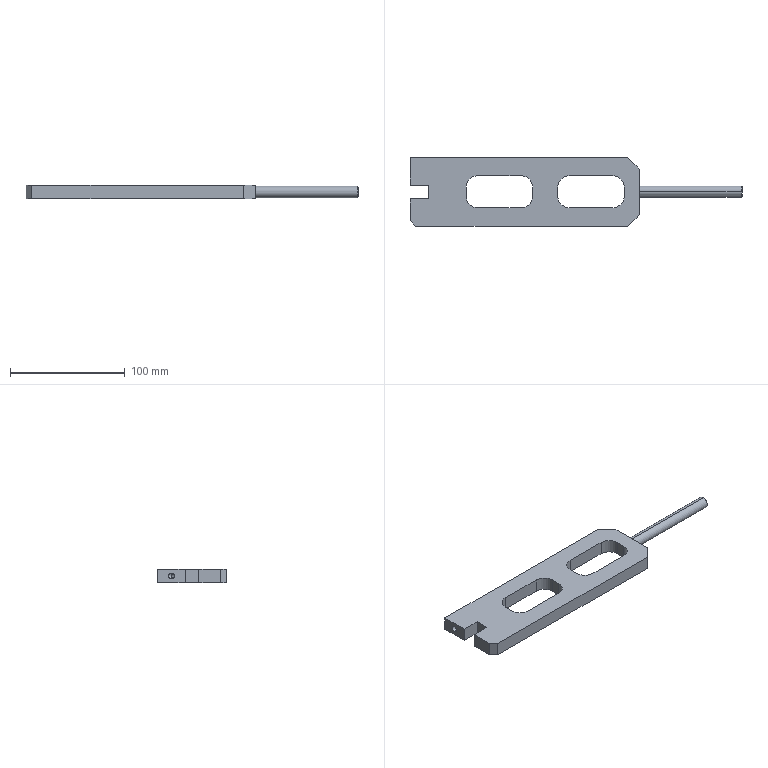Part | SolidWorks | features Chamfer 3, ICE 3, HoleWzd 2, Extrusion 1, Fillet 1, Revolution 1 | 1 solid | 41 faces | box 289.75 x 60 x 12 mm | volume 104525 mm3 | plane 21 | cylinder 14 | cone 6 | commonest cylinder face diameters 20 x8 5 x2 8.5 x2 10 x2
STEP:
#1=CARTESIAN_POINT('',(90.5,0.2,4.25));
#2=VERTEX_POINT('',#1);
#3=CARTESIAN_POINT('',(90.5,0.2,-4.25));
#4=VERTEX_POINT('',#3);
#5=CARTESIAN_POINT('',(90.5,0.2,0.));
#6=DIRECTION('',(1.,0.,0.));
#7=DIRECTION('',(0.,0.,-1.));
#8=AXIS2_PLACEMENT_3D('',#5,#6,#7);
#9=CIRCLE('',#8,4.25);
#10=EDGE_CURVE('',#2,#4,#9,.T.);
#11=ORIENTED_EDGE('',*,*,#10,.F.);
#12=CARTESIAN_POINT('',(189.75,0.2,4.25));
#13=VERTEX_POINT('',#12);
#14=CARTESIAN_POINT('',(190.,0.2,4.25));
#15=DIRECTION('',(1.,0.,0.));
#16=VECTOR('',#15,1000.);
#17=LINE('',#14,#16);
#18=EDGE_CURVE('',#2,#13,#17,.T.);
#19=ORIENTED_EDGE('',*,*,#18,.T.);
#20=CARTESIAN_POINT('',(189.75,0.2,-4.25));
#21=VERTEX_POINT('',#20);
#22=CARTESIAN_POINT('',(189.75,0.2,0.));
#23=DIRECTION('',(1.,0.,0.));
#24=DIRECTION('',(0.,0.,1.));
#25=AXIS2_PLACEMENT_3D('',#22,#23,#24);
#26=CIRCLE('',#25,4.25);
#27=EDGE_CURVE('',#13,#21,#26,.T.);
#28=ORIENTED_EDGE('',*,*,#27,.T.);
#29=CARTESIAN_POINT('',(190.,0.2,-4.25));
#30=DIRECTION('',(1.,0.,0.));
#31=VECTOR('',#30,1000.);
#32=LINE('',#29,#31);
#33=EDGE_CURVE('',#4,#21,#32,.T.);
#34=ORIENTED_EDGE('',*,*,#33,.F.);
#35=EDGE_LOOP('',(#11,#19,#28,#34));
#36=FACE_OUTER_BOUND('',#35,.T.);
#37=CARTESIAN_POINT('',(190.,0.2,0.));
#38=DIRECTION('',(1.,0.,0.));
#39=DIRECTION('',(0.,0.,-1.));
#40=AXIS2_PLACEMENT_3D('',#37,#38,#39);
#41=CYLINDRICAL_SURFACE('',#40,4.25);
#42=ADVANCED_FACE('',(#36),#41,.F.);
#43=CARTESIAN_POINT('',(87.946,0.2,0.));
#44=VERTEX_POINT('',#43);
#45=CARTESIAN_POINT('',(90.5,0.2,-4.25));
#46=DIRECTION('',(0.515,0.,-0.8572));
#47=VECTOR('',#46,1000.);
#48=LINE('',#45,#47);
#49=EDGE_CURVE('',#44,#4,#48,.T.);
#50=ORIENTED_EDGE('',*,*,#49,.F.);
#51=CARTESIAN_POINT('',(90.5,0.2,4.25));
#52=DIRECTION('',(0.515,0.,0.8572));
#53=VECTOR('',#52,1000.);
#54=LINE('',#51,#53);
#55=EDGE_CURVE('',#44,#2,#54,.T.);
#56=ORIENTED_EDGE('',*,*,#55,.T.);
#57=ORIENTED_EDGE('',*,*,#10,.T.);
#58=EDGE_LOOP('',(#50,#56,#57));
#59=FACE_OUTER_BOUND('',#58,.T.);
#60=CARTESIAN_POINT('',(90.5,0.2,0.));
#61=DIRECTION('',(1.,0.,0.));
#62=DIRECTION('',(0.,0.,-1.));
#63=AXIS2_PLACEMENT_3D('',#60,#61,#62);
#64=CONICAL_SURFACE('',#63,4.25,1.03);
#65=ADVANCED_FACE('',(#59),#64,.F.);
#66=CARTESIAN_POINT('',(189.75,0.2,0.));
#67=DIRECTION('',(1.,0.,0.));
#68=DIRECTION('',(0.,0.,1.));
#69=AXIS2_PLACEMENT_3D('',#66,#67,#68);
#70=CIRCLE('',#69,4.25);
#71=EDGE_CURVE('',#21,#13,#70,.T.);
#72=ORIENTED_EDGE('',*,*,#71,.F.);
#73=CARTESIAN_POINT('',(189.,0.2,-5.));
#74=VERTEX_POINT('',#73);
#75=CARTESIAN_POINT('',(189.,0.2,-5.));
#76=DIRECTION('',(-0.7071,0.,-0.7071));
#77=VECTOR('',#76,1000.);
#78=LINE('',#75,#77);
#79=EDGE_CURVE('',#21,#74,#78,.T.);
#80=ORIENTED_EDGE('',*,*,#79,.T.);
#81=CARTESIAN_POINT('',(189.,0.2,5.));
#82=VERTEX_POINT('',#81);
#83=CARTESIAN_POINT('',(189.,0.2,0.));
#84=DIRECTION('',(-1.,0.,0.));
#85=DIRECTION('',(0.,0.,-1.));
#86=AXIS2_PLACEMENT_3D('',#83,#84,#85);
#87=CIRCLE('',#86,5.);
#88=EDGE_CURVE('',#82,#74,#87,.T.);
#89=ORIENTED_EDGE('',*,*,#88,.F.);
#90=CARTESIAN_POINT('',(189.,0.2,5.));
#91=DIRECTION('',(-0.7071,0.,0.7071));
#92=VECTOR('',#91,1000.);
#93=LINE('',#90,#92);
#94=EDGE_CURVE('',#13,#82,#93,.T.);
#95=ORIENTED_EDGE('',*,*,#94,.F.);
#96=EDGE_LOOP('',(#72,#80,#89,#95));
#97=FACE_OUTER_BOUND('',#96,.T.);
#98=CARTESIAN_POINT('',(189.,0.2,0.));
#99=DIRECTION('',(-1.,0.,0.));
#100=DIRECTION('',(0.,0.,1.));
#101=AXIS2_PLACEMENT_3D('',#98,#99,#100);
#102=CONICAL_SURFACE('',#101,5.,0.7854);
#103=ADVANCED_FACE('',(#97),#102,.T.);
#104=CARTESIAN_POINT('',(-87.,18.,-2.5));
#105=VERTEX_POINT('',#104);
#106=CARTESIAN_POINT('',(-87.,18.,2.5));
#107=VERTEX_POINT('',#106);
#108=CARTESIAN_POINT('',(-87.,18.,0.));
#109=DIRECTION('',(-1.,0.,0.));
#110=DIRECTION('',(0.,0.,1.));
#111=AXIS2_PLACEMENT_3D('',#108,#109,#110);
#112=CIRCLE('',#111,2.5);
#113=EDGE_CURVE('',#105,#107,#112,.T.);
#114=ORIENTED_EDGE('',*,*,#113,.F.);
#115=CARTESIAN_POINT('',(-100.,18.,-2.5));
#116=VERTEX_POINT('',#115);
#117=CARTESIAN_POINT('',(-100.,18.,-2.5));
#118=DIRECTION('',(-1.,0.,0.));
#119=VECTOR('',#118,1000.);
#120=LINE('',#117,#119);
#121=EDGE_CURVE('',#105,#116,#120,.T.);
#122=ORIENTED_EDGE('',*,*,#121,.T.);
#123=CARTESIAN_POINT('',(-100.,18.,2.5));
#124=VERTEX_POINT('',#123);
#125=CARTESIAN_POINT('',(-100.,18.,0.));
#126=DIRECTION('',(-1.,0.,0.));
#127=DIRECTION('',(0.,0.,1.));
#128=AXIS2_PLACEMENT_3D('',#125,#126,#127);
#129=CIRCLE('',#128,2.5);
#130=EDGE_CURVE('',#116,#124,#129,.T.);
#131=ORIENTED_EDGE('',*,*,#130,.T.);
#132=CARTESIAN_POINT('',(-100.,18.,2.5));
#133=DIRECTION('',(-1.,0.,0.));
#134=VECTOR('',#133,1000.);
#135=LINE('',#132,#134);
#136=EDGE_CURVE('',#107,#124,#135,.T.);
#137=ORIENTED_EDGE('',*,*,#136,.F.);
#138=EDGE_LOOP('',(#114,#122,#131,#137));
#139=FACE_OUTER_BOUND('',#138,.T.);
#140=CARTESIAN_POINT('',(-100.,18.,0.));
#141=DIRECTION('',(-1.,0.,0.));
#142=DIRECTION('',(0.,0.,1.));
#143=AXIS2_PLACEMENT_3D('',#140,#141,#142);
#144=CYLINDRICAL_SURFACE('',#143,2.5);
#145=ADVANCED_FACE('',(#139),#144,.F.);
#146=CARTESIAN_POINT('',(-85.498,18.,0.));
#147=VERTEX_POINT('',#146);
#148=CARTESIAN_POINT('',(-87.,18.,2.5));
#149=DIRECTION('',(-0.515,0.,0.8572));
#150=VECTOR('',#149,1000.);
#151=LINE('',#148,#150);
#152=EDGE_CURVE('',#147,#107,#151,.T.);
#153=ORIENTED_EDGE('',*,*,#152,.F.);
#154=CARTESIAN_POINT('',(-87.,18.,-2.5));
#155=DIRECTION('',(-0.515,0.,-0.8572));
#156=VECTOR('',#155,1000.);
#157=LINE('',#154,#156);
#158=EDGE_CURVE('',#147,#105,#157,.T.);
#159=ORIENTED_EDGE('',*,*,#158,.T.);
#160=ORIENTED_EDGE('',*,*,#113,.T.);
#161=EDGE_LOOP('',(#153,#159,#160));
#162=FACE_OUTER_BOUND('',#161,.T.);
#163=CARTESIAN_POINT('',(-87.,18.,0.));
#164=DIRECTION('',(-1.,0.,0.));
#165=DIRECTION('',(0.,0.,1.));
#166=AXIS2_PLACEMENT_3D('',#163,#164,#165);
#167=CONICAL_SURFACE('',#166,2.5,1.03);
#168=ADVANCED_FACE('',(#162),#167,.F.);
#169=ORIENTED_EDGE('',*,*,#88,.T.);
#170=CARTESIAN_POINT('',(100.,0.2,-5.));
#171=VERTEX_POINT('',#170);
#172=CARTESIAN_POINT('',(190.,0.2,-5.));
#173=DIRECTION('',(-1.,0.,0.));
#174=VECTOR('',#173,1000.);
#175=LINE('',#172,#174);
#176=EDGE_CURVE('',#74,#171,#175,.T.);
#177=ORIENTED_EDGE('',*,*,#176,.T.);
#178=CARTESIAN_POINT('',(100.,0.2,5.));
#179=VERTEX_POINT('',#178);
#180=CARTESIAN_POINT('',(100.,0.2,0.));
#181=DIRECTION('',(-1.,0.,0.));
#182=DIRECTION('',(0.,0.,1.));
#183=AXIS2_PLACEMENT_3D('',#180,#181,#182);
#184=CIRCLE('',#183,5.);
#185=EDGE_CURVE('',#179,#171,#184,.T.);
#186=ORIENTED_EDGE('',*,*,#185,.F.);
#187=CARTESIAN_POINT('',(190.,0.2,5.));
#188=DIRECTION('',(-1.,0.,0.));
#189=VECTOR('',#188,1000.);
#190=LINE('',#187,#189);
#191=EDGE_CURVE('',#82,#179,#190,.T.);
#192=ORIENTED_EDGE('',*,*,#191,.F.);
#193=EDGE_LOOP('',(#169,#177,#186,#192));
#194=FACE_OUTER_BOUND('',#193,.T.);
#195=CARTESIAN_POINT('',(190.,0.2,0.));
#196=DIRECTION('',(-1.,0.,0.));
#197=DIRECTION('',(0.,0.,1.));
#198=AXIS2_PLACEMENT_3D('',#195,#196,#197);
#199=CYLINDRICAL_SURFACE('',#198,5.);
#200=ADVANCED_FACE('',(#194),#199,.T.);
#201=CARTESIAN_POINT('',(-100.,-6.,-6.));
#202=VERTEX_POINT('',#201);
#203=CARTESIAN_POINT('',(-100.,-25.,-6.));
#204=VERTEX_POINT('',#203);
#205=CARTESIAN_POINT('',(-100.,30.,-6.));
#206=DIRECTION('',(0.,-1.,0.));
#207=VECTOR('',#206,1000.);
#208=LINE('',#205,#207);
#209=EDGE_CURVE('',#202,#204,#208,.T.);
#210=ORIENTED_EDGE('',*,*,#209,.T.);
#211=CARTESIAN_POINT('',(-100.,-25.,6.));
#212=VERTEX_POINT('',#211);
#213=CARTESIAN_POINT('',(-100.,-25.,-6.));
#214=DIRECTION('',(0.,0.,1.));
#215=VECTOR('',#214,1000.);
#216=LINE('',#213,#215);
#217=EDGE_CURVE('',#204,#212,#216,.T.);
#218=ORIENTED_EDGE('',*,*,#217,.T.);
#219=CARTESIAN_POINT('',(-100.,-6.,6.));
#220=VERTEX_POINT('',#219);
#221=CARTESIAN_POINT('',(-100.,30.,6.));
#222=DIRECTION('',(0.,-1.,0.));
#223=VECTOR('',#222,1000.);
#224=LINE('',#221,#223);
#225=EDGE_CURVE('',#220,#212,#224,.T.);
#226=ORIENTED_EDGE('',*,*,#225,.F.);
#227=CARTESIAN_POINT('',(-100.,-6.,6.));
#228=DIRECTION('',(0.,0.,-1.));
#229=VECTOR('',#228,1000.);
#230=LINE('',#227,#229);
#231=EDGE_CURVE('',#220,#202,#230,.T.);
#232=ORIENTED_EDGE('',*,*,#231,.T.);
#233=EDGE_LOOP('',(#210,#218,#226,#232));
#234=FACE_OUTER_BOUND('',#233,.T.);
#235=CARTESIAN_POINT('',(-100.,30.,-6.));
#236=DIRECTION('',(-1.,0.,0.));
#237=DIRECTION('',(0.,0.,1.));
#238=AXIS2_PLACEMENT_3D('',#235,#236,#237);
#239=PLANE('',#238);
#240=ADVANCED_FACE('',(#234),#239,.T.);
#241=CARTESIAN_POINT('',(90.,30.,6.));
#242=VERTEX_POINT('',#241);
#243=CARTESIAN_POINT('',(-100.,30.,6.));
#244=VERTEX_POINT('',#243);
#245=CARTESIAN_POINT('',(100.,30.,6.));
#246=DIRECTION('',(-1.,0.,0.));
#247=VECTOR('',#246,1000.);
#248=LINE('',#245,#247);
#249=EDGE_CURVE('',#242,#244,#248,.T.);
#250=ORIENTED_EDGE('',*,*,#249,.F.);
#251=CARTESIAN_POINT('',(90.,30.,-6.));
#252=VERTEX_POINT('',#251);
#253=CARTESIAN_POINT('',(90.,30.,-6.));
#254=DIRECTION('',(0.,0.,-1.));
#255=VECTOR('',#254,1000.);
#256=LINE('',#253,#255);
#257=EDGE_CURVE('',#242,#252,#256,.T.);
#258=ORIENTED_EDGE('',*,*,#257,.T.);
#259=CARTESIAN_POINT('',(-100.,30.,-6.));
#260=VERTEX_POINT('',#259);
#261=CARTESIAN_POINT('',(100.,30.,-6.));
#262=DIRECTION('',(-1.,0.,0.));
#263=VECTOR('',#262,1000.);
#264=LINE('',#261,#263);
#265=EDGE_CURVE('',#252,#260,#264,.T.);
#266=ORIENTED_EDGE('',*,*,#265,.T.);
#267=CARTESIAN_POINT('',(-100.,30.,-6.));
#268=DIRECTION('',(0.,0.,1.));
#269=VECTOR('',#268,1000.);
#270=LINE('',#267,#269);
#271=EDGE_CURVE('',#260,#244,#270,.T.);
#272=ORIENTED_EDGE('',*,*,#271,.T.);
#273=EDGE_LOOP('',(#250,#258,#266,#272));
#274=FACE_OUTER_BOUND('',#273,.T.);
#275=CARTESIAN_POINT('',(100.,30.,-6.));
#276=DIRECTION('',(0.,1.,0.));
#277=DIRECTION('',(0.,0.,1.));
#278=AXIS2_PLACEMENT_3D('',#275,#276,#277);
#279=PLANE('',#278);
#280=ADVANCED_FACE('',(#274),#279,.T.);
#281=ORIENTED_EDGE('',*,*,#185,.T.);
#282=CARTESIAN_POINT('',(100.,0.2,0.));
#283=DIRECTION('',(-1.,0.,0.));
#284=DIRECTION('',(0.,0.,1.));
#285=AXIS2_PLACEMENT_3D('',#282,#283,#284);
#286=CIRCLE('',#285,5.);
#287=EDGE_CURVE('',#171,#179,#286,.T.);
#288=ORIENTED_EDGE('',*,*,#287,.T.);
#289=EDGE_LOOP('',(#281,#288));
#290=FACE_BOUND('',#289,.T.);
#291=CARTESIAN_POINT('',(100.,-20.,-6.));
#292=VERTEX_POINT('',#291);
#293=CARTESIAN_POINT('',(100.,20.,-6.));
#294=VERTEX_POINT('',#293);
#295=CARTESIAN_POINT('',(100.,-30.,-6.));
#296=DIRECTION('',(0.,1.,0.));
#297=VECTOR('',#296,1000.);
#298=LINE('',#295,#297);
#299=EDGE_CURVE('',#292,#294,#298,.T.);
#300=ORIENTED_EDGE('',*,*,#299,.T.);
#301=CARTESIAN_POINT('',(100.,20.,6.));
#302=VERTEX_POINT('',#301);
#303=CARTESIAN_POINT('',(100.,20.,-6.));
#304=DIRECTION('',(0.,0.,1.));
#305=VECTOR('',#304,1000.);
#306=LINE('',#303,#305);
#307=EDGE_CURVE('',#294,#302,#306,.T.);
#308=ORIENTED_EDGE('',*,*,#307,.T.);
#309=CARTESIAN_POINT('',(100.,-20.,6.));
#310=VERTEX_POINT('',#309);
#311=CARTESIAN_POINT('',(100.,-30.,6.));
#312=DIRECTION('',(0.,1.,0.));
#313=VECTOR('',#312,1000.);
#314=LINE('',#311,#313);
#315=EDGE_CURVE('',#310,#302,#314,.T.);
#316=ORIENTED_EDGE('',*,*,#315,.F.);
#317=CARTESIAN_POINT('',(100.,-20.,-6.));
#318=DIRECTION('',(0.,0.,-1.));
#319=VECTOR('',#318,1000.);
#320=LINE('',#317,#319);
#321=EDGE_CURVE('',#310,#292,#320,.T.);
#322=ORIENTED_EDGE('',*,*,#321,.T.);
#323=EDGE_LOOP('',(#300,#308,#316,#322));
#324=FACE_OUTER_BOUND('',#323,.T.);
#325=CARTESIAN_POINT('',(100.,-30.,-6.));
#326=DIRECTION('',(1.,0.,0.));
#327=DIRECTION('',(0.,0.,-1.));
#328=AXIS2_PLACEMENT_3D('',#325,#326,#327);
#329=PLANE('',#328);
#330=ADVANCED_FACE('',(#290,#324),#329,.T.);
#331=CARTESIAN_POINT('',(-95.,-30.,6.));
#332=VERTEX_POINT('',#331);
#333=CARTESIAN_POINT('',(90.,-30.,6.));
#334=VERTEX_POINT('',#333);
#335=CARTESIAN_POINT('',(-100.,-30.,6.));
#336=DIRECTION('',(1.,0.,0.));
#337=VECTOR('',#336,1000.);
#338=LINE('',#335,#337);
#339=EDGE_CURVE('',#332,#334,#338,.T.);
#340=ORIENTED_EDGE('',*,*,#339,.F.);
#341=CARTESIAN_POINT('',(-95.,-30.,-6.));
#342=VERTEX_POINT('',#341);
#343=CARTESIAN_POINT('',(-95.,-30.,-6.));
#344=DIRECTION('',(0.,0.,-1.));
#345=VECTOR('',#344,1000.);
#346=LINE('',#343,#345);
#347=EDGE_CURVE('',#332,#342,#346,.T.);
#348=ORIENTED_EDGE('',*,*,#347,.T.);
#349=CARTESIAN_POINT('',(90.,-30.,-6.));
#350=VERTEX_POINT('',#349);
#351=CARTESIAN_POINT('',(-100.,-30.,-6.));
#352=DIRECTION('',(1.,0.,0.));
#353=VECTOR('',#352,1000.);
#354=LINE('',#351,#353);
#355=EDGE_CURVE('',#342,#350,#354,.T.);
#356=ORIENTED_EDGE('',*,*,#355,.T.);
#357=CARTESIAN_POINT('',(90.,-30.,-6.));
#358=DIRECTION('',(0.,0.,1.));
#359=VECTOR('',#358,1000.);
#360=LINE('',#357,#359);
#361=EDGE_CURVE('',#350,#334,#360,.T.);
#362=ORIENTED_EDGE('',*,*,#361,.T.);
#363=EDGE_LOOP('',(#340,#348,#356,#362));
#364=FACE_OUTER_BOUND('',#363,.T.);
#365=CARTESIAN_POINT('',(-100.,-30.,-6.));
#366=DIRECTION('',(0.,-1.,0.));
#367=DIRECTION('',(0.,0.,-1.));
#368=AXIS2_PLACEMENT_3D('',#365,#366,#367);
#369=PLANE('',#368);
#370=ADVANCED_FACE('',(#364),#369,.T.);
#371=CARTESIAN_POINT('',(-100.,18.,0.));
#372=DIRECTION('',(-1.,0.,0.));
#373=DIRECTION('',(0.,0.,1.));
#374=AXIS2_PLACEMENT_3D('',#371,#372,#373);
#375=CIRCLE('',#374,2.5);
#376=EDGE_CURVE('',#124,#116,#375,.T.);
#377=ORIENTED_EDGE('',*,*,#376,.F.);
#378=ORIENTED_EDGE('',*,*,#130,.F.);
#379=EDGE_LOOP('',(#377,#378));
#380=FACE_BOUND('',#379,.T.);
#381=CARTESIAN_POINT('',(-100.,6.,6.));
#382=VERTEX_POINT('',#381);
#383=CARTESIAN_POINT('',(-100.,6.,-6.));
#384=VERTEX_POINT('',#383);
#385=CARTESIAN_POINT('',(-100.,6.,6.));
#386=DIRECTION('',(0.,0.,-1.));
#387=VECTOR('',#386,1000.);
#388=LINE('',#385,#387);
#389=EDGE_CURVE('',#382,#384,#388,.T.);
#390=ORIENTED_EDGE('',*,*,#389,.F.);
#391=CARTESIAN_POINT('',(-100.,30.,6.));
#392=DIRECTION('',(0.,-1.,0.));
#393=VECTOR('',#392,1000.);
#394=LINE('',#391,#393);
#395=EDGE_CURVE('',#244,#382,#394,.T.);
#396=ORIENTED_EDGE('',*,*,#395,.F.);
#397=ORIENTED_EDGE('',*,*,#271,.F.);
#398=CARTESIAN_POINT('',(-100.,30.,-6.));
#399=DIRECTION('',(0.,-1.,0.));
#400=VECTOR('',#399,1000.);
#401=LINE('',#398,#400);
#402=EDGE_CURVE('',#260,#384,#401,.T.);
#403=ORIENTED_EDGE('',*,*,#402,.T.);
#404=EDGE_LOOP('',(#390,#396,#397,#403));
#405=FACE_OUTER_BOUND('',#404,.T.);
#406=CARTESIAN_POINT('',(-100.,30.,-6.));
#407=DIRECTION('',(-1.,0.,0.));
#408=DIRECTION('',(0.,0.,1.));
#409=AXIS2_PLACEMENT_3D('',#406,#407,#408);
#410=PLANE('',#409);
#411=ADVANCED_FACE('',(#380,#405),#410,.T.);
#412=CARTESIAN_POINT('',(39.,14.2,-6.));
#413=VERTEX_POINT('',#412);
#414=CARTESIAN_POINT('',(77.,14.2,-6.));
#415=VERTEX_POINT('',#414);
#416=CARTESIAN_POINT('',(29.,14.2,-6.));
#417=DIRECTION('',(1.,0.,0.));
#418=VECTOR('',#417,1000.);
#419=LINE('',#416,#418);
#420=EDGE_CURVE('',#413,#415,#419,.T.);
#421=ORIENTED_EDGE('',*,*,#420,.F.);
#422=CARTESIAN_POINT('',(29.,4.2,-6.));
#423=VERTEX_POINT('',#422);
#424=CARTESIAN_POINT('',(39.,4.2,-6.));
#425=DIRECTION('',(0.,0.,1.));
#426=DIRECTION('',(1.,0.,0.));
#427=AXIS2_PLACEMENT_3D('',#424,#425,#426);
#428=CIRCLE('',#427,10.);
#429=EDGE_CURVE('',#413,#423,#428,.T.);
#430=ORIENTED_EDGE('',*,*,#429,.T.);
#431=CARTESIAN_POINT('',(29.,-3.8,-6.));
#432=VERTEX_POINT('',#431);
#433=CARTESIAN_POINT('',(29.,-13.8,-6.));
#434=DIRECTION('',(0.,1.,0.));
#435=VECTOR('',#434,1000.);
#436=LINE('',#433,#435);
#437=EDGE_CURVE('',#432,#423,#436,.T.);
#438=ORIENTED_EDGE('',*,*,#437,.F.);
#439=CARTESIAN_POINT('',(39.,-13.8,-6.));
#440=VERTEX_POINT('',#439);
#441=CARTESIAN_POINT('',(39.,-3.8,-6.));
#442=DIRECTION('',(0.,0.,1.));
#443=DIRECTION('',(1.,0.,0.));
#444=AXIS2_PLACEMENT_3D('',#441,#442,#443);
#445=CIRCLE('',#444,10.);
#446=EDGE_CURVE('',#432,#440,#445,.T.);
#447=ORIENTED_EDGE('',*,*,#446,.T.);
#448=CARTESIAN_POINT('',(77.,-13.8,-6.));
#449=VERTEX_POINT('',#448);
#450=CARTESIAN_POINT('',(87.,-13.8,-6.));
#451=DIRECTION('',(-1.,0.,0.));
#452=VECTOR('',#451,1000.);
#453=LINE('',#450,#452);
#454=EDGE_CURVE('',#449,#440,#453,.T.);
#455=ORIENTED_EDGE('',*,*,#454,.F.);
#456=CARTESIAN_POINT('',(87.,-3.8,-6.));
#457=VERTEX_POINT('',#456);
#458=CARTESIAN_POINT('',(77.,-3.8,-6.));
#459=DIRECTION('',(0.,0.,1.));
#460=DIRECTION('',(1.,0.,0.));
#461=AXIS2_PLACEMENT_3D('',#458,#459,#460);
#462=CIRCLE('',#461,10.);
#463=EDGE_CURVE('',#449,#457,#462,.T.);
#464=ORIENTED_EDGE('',*,*,#463,.T.);
#465=CARTESIAN_POINT('',(87.,4.2,-6.));
#466=VERTEX_POINT('',#465);
#467=CARTESIAN_POINT('',(87.,14.2,-6.));
#468=DIRECTION('',(0.,-1.,0.));
#469=VECTOR('',#468,1000.);
#470=LINE('',#467,#469);
#471=EDGE_CURVE('',#466,#457,#470,.T.);
#472=ORIENTED_EDGE('',*,*,#471,.F.);
#473=CARTESIAN_POINT('',(77.,4.2,-6.));
#474=DIRECTION('',(0.,0.,1.));
#475=DIRECTION('',(1.,0.,0.));
#476=AXIS2_PLACEMENT_3D('',#473,#474,#475);
#477=CIRCLE('',#476,10.);
#478=EDGE_CURVE('',#466,#415,#477,.T.);
#479=ORIENTED_EDGE('',*,*,#478,.T.);
#480=EDGE_LOOP('',(#421,#430,#438,#447,#455,#464,#472,#479));
#481=FACE_BOUND('',#480,.T.);
#482=CARTESIAN_POINT('',(7.,-3.8,-6.));
#483=VERTEX_POINT('',#482);
#484=CARTESIAN_POINT('',(7.,4.2,-6.));
#485=VERTEX_POINT('',#484);
#486=CARTESIAN_POINT('',(7.,-13.8,-6.));
#487=DIRECTION('',(0.,1.,0.));
#488=VECTOR('',#487,1000.);
#489=LINE('',#486,#488);
#490=EDGE_CURVE('',#483,#485,#489,.T.);
#491=ORIENTED_EDGE('',*,*,#490,.T.);
#492=CARTESIAN_POINT('',(-3.,14.2,-6.));
#493=VERTEX_POINT('',#492);
#494=CARTESIAN_POINT('',(-3.,4.2,-6.));
#495=DIRECTION('',(0.,0.,1.));
#496=DIRECTION('',(1.,0.,0.));
#497=AXIS2_PLACEMENT_3D('',#494,#495,#496);
#498=CIRCLE('',#497,10.);
#499=EDGE_CURVE('',#485,#493,#498,.T.);
#500=ORIENTED_EDGE('',*,*,#499,.T.);
#501=CARTESIAN_POINT('',(-41.,14.2,-6.));
#502=VERTEX_POINT('',#501);
#503=CARTESIAN_POINT('',(7.,14.2,-6.));
#504=DIRECTION('',(-1.,0.,0.));
#505=VECTOR('',#504,1000.);
#506=LINE('',#503,#505);
#507=EDGE_CURVE('',#493,#502,#506,.T.);
#508=ORIENTED_EDGE('',*,*,#507,.T.);
#509=CARTESIAN_POINT('',(-51.,4.2,-6.));
#510=VERTEX_POINT('',#509);
#511=CARTESIAN_POINT('',(-41.,4.2,-6.));
#512=DIRECTION('',(0.,0.,1.));
#513=DIRECTION('',(1.,0.,0.));
#514=AXIS2_PLACEMENT_3D('',#511,#512,#513);
#515=CIRCLE('',#514,10.);
#516=EDGE_CURVE('',#502,#510,#515,.T.);
#517=ORIENTED_EDGE('',*,*,#516,.T.);
#518=CARTESIAN_POINT('',(-51.,-3.8,-6.));
#519=VERTEX_POINT('',#518);
#520=CARTESIAN_POINT('',(-51.,14.2,-6.));
#521=DIRECTION('',(0.,-1.,0.));
#522=VECTOR('',#521,1000.);
#523=LINE('',#520,#522);
#524=EDGE_CURVE('',#510,#519,#523,.T.);
#525=ORIENTED_EDGE('',*,*,#524,.T.);
#526=CARTESIAN_POINT('',(-41.,-13.8,-6.));
#527=VERTEX_POINT('',#526);
#528=CARTESIAN_POINT('',(-41.,-3.8,-6.));
#529=DIRECTION('',(0.,0.,1.));
#530=DIRECTION('',(1.,0.,0.));
#531=AXIS2_PLACEMENT_3D('',#528,#529,#530);
#532=CIRCLE('',#531,10.);
#533=EDGE_CURVE('',#519,#527,#532,.T.);
#534=ORIENTED_EDGE('',*,*,#533,.T.);
#535=CARTESIAN_POINT('',(-3.,-13.8,-6.));
#536=VERTEX_POINT('',#535);
#537=CARTESIAN_POINT('',(-51.,-13.8,-6.));
#538=DIRECTION('',(1.,0.,0.));
#539=VECTOR('',#538,1000.);
#540=LINE('',#537,#539);
#541=EDGE_CURVE('',#527,#536,#540,.T.);
#542=ORIENTED_EDGE('',*,*,#541,.T.);
#543=CARTESIAN_POINT('',(-3.,-3.8,-6.));
#544=DIRECTION('',(0.,0.,1.));
#545=DIRECTION('',(1.,0.,0.));
#546=AXIS2_PLACEMENT_3D('',#543,#544,#545);
#547=CIRCLE('',#546,10.);
#548=EDGE_CURVE('',#536,#483,#547,.T.);
#549=ORIENTED_EDGE('',*,*,#548,.T.);
#550=EDGE_LOOP('',(#491,#500,#508,#517,#525,#534,#542,#549));
#551=FACE_BOUND('',#550,.T.);
#552=ORIENTED_EDGE('',*,*,#355,.F.);
#553=CARTESIAN_POINT('',(-100.,-25.,-6.));
#554=DIRECTION('',(-0.7071,0.7071,0.));
#555=VECTOR('',#554,1000.);
#556=LINE('',#553,#555);
#557=EDGE_CURVE('',#342,#204,#556,.T.);
#558=ORIENTED_EDGE('',*,*,#557,.T.);
#559=ORIENTED_EDGE('',*,*,#209,.F.);
#560=CARTESIAN_POINT('',(-84.,-6.,-6.));
#561=VERTEX_POINT('',#560);
#562=CARTESIAN_POINT('',(-84.,-6.,-6.));
#563=DIRECTION('',(-1.,0.,0.));
#564=VECTOR('',#563,1000.);
#565=LINE('',#562,#564);
#566=EDGE_CURVE('',#561,#202,#565,.T.);
#567=ORIENTED_EDGE('',*,*,#566,.F.);
#568=CARTESIAN_POINT('',(-84.,6.,-6.));
#569=VERTEX_POINT('',#568);
#570=CARTESIAN_POINT('',(-84.,6.,-6.));
#571=DIRECTION('',(0.,-1.,0.));
#572=VECTOR('',#571,1000.);
#573=LINE('',#570,#572);
#574=EDGE_CURVE('',#569,#561,#573,.T.);
#575=ORIENTED_EDGE('',*,*,#574,.F.);
#576=CARTESIAN_POINT('',(-100.,6.,-6.));
#577=DIRECTION('',(1.,0.,0.));
#578=VECTOR('',#577,1000.);
#579=LINE('',#576,#578);
#580=EDGE_CURVE('',#384,#569,#579,.T.);
#581=ORIENTED_EDGE('',*,*,#580,.F.);
#582=ORIENTED_EDGE('',*,*,#402,.F.);
#583=ORIENTED_EDGE('',*,*,#265,.F.);
#584=CARTESIAN_POINT('',(100.,20.,-6.));
#585=DIRECTION('',(0.7071,-0.7071,0.));
#586=VECTOR('',#585,1000.);
#587=LINE('',#584,#586);
#588=EDGE_CURVE('',#252,#294,#587,.T.);
#589=ORIENTED_EDGE('',*,*,#588,.T.);
#590=ORIENTED_EDGE('',*,*,#299,.F.);
#591=CARTESIAN_POINT('',(90.,-30.,-6.));
#592=DIRECTION('',(-0.7071,-0.7071,0.));
#593=VECTOR('',#592,1000.);
#594=LINE('',#591,#593);
#595=EDGE_CURVE('',#292,#350,#594,.T.);
#596=ORIENTED_EDGE('',*,*,#595,.T.);
#597=EDGE_LOOP('',(#552,#558,#559,#567,#575,#581,#582,#583,#589,#590,#596));
#598=FACE_OUTER_BOUND('',#597,.T.);
#599=CARTESIAN_POINT('',(0.,0.,-6.));
#600=DIRECTION('',(0.,0.,1.));
#601=DIRECTION('',(1.,0.,0.));
#602=AXIS2_PLACEMENT_3D('',#599,#600,#601);
#603=PLANE('',#602);
#604=ADVANCED_FACE('',(#481,#551,#598),#603,.F.);
#605=CARTESIAN_POINT('',(77.,-13.8,6.));
#606=VERTEX_POINT('',#605);
#607=CARTESIAN_POINT('',(39.,-13.8,6.));
#608=VERTEX_POINT('',#607);
#609=CARTESIAN_POINT('',(87.,-13.8,6.));
#610=DIRECTION('',(-1.,0.,0.));
#611=VECTOR('',#610,1000.);
#612=LINE('',#609,#611);
#613=EDGE_CURVE('',#606,#608,#612,.T.);
#614=ORIENTED_EDGE('',*,*,#613,.T.);
#615=CARTESIAN_POINT('',(29.,-3.8,6.));
#616=VERTEX_POINT('',#615);
#617=CARTESIAN_POINT('',(39.,-3.8,6.));
#618=DIRECTION('',(0.,0.,-1.));
#619=DIRECTION('',(1.,0.,0.));
#620=AXIS2_PLACEMENT_3D('',#617,#618,#619);
#621=CIRCLE('',#620,10.);
#622=EDGE_CURVE('',#608,#616,#621,.T.);
#623=ORIENTED_EDGE('',*,*,#622,.T.);
#624=CARTESIAN_POINT('',(29.,4.2,6.));
#625=VERTEX_POINT('',#624);
#626=CARTESIAN_POINT('',(29.,-13.8,6.));
#627=DIRECTION('',(0.,1.,0.));
#628=VECTOR('',#627,1000.);
#629=LINE('',#626,#628);
#630=EDGE_CURVE('',#616,#625,#629,.T.);
#631=ORIENTED_EDGE('',*,*,#630,.T.);
#632=CARTESIAN_POINT('',(39.,14.2,6.));
#633=VERTEX_POINT('',#632);
#634=CARTESIAN_POINT('',(39.,4.2,6.));
#635=DIRECTION('',(0.,0.,-1.));
#636=DIRECTION('',(1.,0.,0.));
#637=AXIS2_PLACEMENT_3D('',#634,#635,#636);
#638=CIRCLE('',#637,10.);
#639=EDGE_CURVE('',#625,#633,#638,.T.);
#640=ORIENTED_EDGE('',*,*,#639,.T.);
#641=CARTESIAN_POINT('',(77.,14.2,6.));
#642=VERTEX_POINT('',#641);
#643=CARTESIAN_POINT('',(29.,14.2,6.));
#644=DIRECTION('',(1.,0.,0.));
#645=VECTOR('',#644,1000.);
#646=LINE('',#643,#645);
#647=EDGE_CURVE('',#633,#642,#646,.T.);
#648=ORIENTED_EDGE('',*,*,#647,.T.);
#649=CARTESIAN_POINT('',(87.,4.2,6.));
#650=VERTEX_POINT('',#649);
#651=CARTESIAN_POINT('',(77.,4.2,6.));
#652=DIRECTION('',(0.,0.,-1.));
#653=DIRECTION('',(1.,0.,0.));
#654=AXIS2_PLACEMENT_3D('',#651,#652,#653);
#655=CIRCLE('',#654,10.);
#656=EDGE_CURVE('',#642,#650,#655,.T.);
#657=ORIENTED_EDGE('',*,*,#656,.T.);
#658=CARTESIAN_POINT('',(87.,-3.8,6.));
#659=VERTEX_POINT('',#658);
#660=CARTESIAN_POINT('',(87.,14.2,6.));
#661=DIRECTION('',(0.,-1.,0.));
#662=VECTOR('',#661,1000.);
#663=LINE('',#660,#662);
#664=EDGE_CURVE('',#650,#659,#663,.T.);
#665=ORIENTED_EDGE('',*,*,#664,.T.);
#666=CARTESIAN_POINT('',(77.,-3.8,6.));
#667=DIRECTION('',(0.,0.,-1.));
#668=DIRECTION('',(1.,0.,0.));
#669=AXIS2_PLACEMENT_3D('',#666,#667,#668);
#670=CIRCLE('',#669,10.);
#671=EDGE_CURVE('',#659,#606,#670,.T.);
#672=ORIENTED_EDGE('',*,*,#671,.T.);
#673=EDGE_LOOP('',(#614,#623,#631,#640,#648,#657,#665,#672));
#674=FACE_BOUND('',#673,.T.);
#675=CARTESIAN_POINT('',(-51.,4.2,6.));
#676=VERTEX_POINT('',#675);
#677=CARTESIAN_POINT('',(-51.,-3.8,6.));
#678=VERTEX_POINT('',#677);
#679=CARTESIAN_POINT('',(-51.,14.2,6.));
#680=DIRECTION('',(0.,-1.,0.));
#681=VECTOR('',#680,1000.);
#682=LINE('',#679,#681);
#683=EDGE_CURVE('',#676,#678,#682,.T.);
#684=ORIENTED_EDGE('',*,*,#683,.F.);
#685=CARTESIAN_POINT('',(-41.,14.2,6.));
#686=VERTEX_POINT('',#685);
#687=CARTESIAN_POINT('',(-41.,4.2,6.));
#688=DIRECTION('',(0.,0.,-1.));
#689=DIRECTION('',(1.,0.,0.));
#690=AXIS2_PLACEMENT_3D('',#687,#688,#689);
#691=CIRCLE('',#690,10.);
#692=EDGE_CURVE('',#676,#686,#691,.T.);
#693=ORIENTED_EDGE('',*,*,#692,.T.);
#694=CARTESIAN_POINT('',(-3.,14.2,6.));
#695=VERTEX_POINT('',#694);
#696=CARTESIAN_POINT('',(7.,14.2,6.));
#697=DIRECTION('',(-1.,0.,0.));
#698=VECTOR('',#697,1000.);
#699=LINE('',#696,#698);
#700=EDGE_CURVE('',#695,#686,#699,.T.);
#701=ORIENTED_EDGE('',*,*,#700,.F.);
#702=CARTESIAN_POINT('',(7.,4.2,6.));
#703=VERTEX_POINT('',#702);
#704=CARTESIAN_POINT('',(-3.,4.2,6.));
#705=DIRECTION('',(0.,0.,-1.));
#706=DIRECTION('',(1.,0.,0.));
#707=AXIS2_PLACEMENT_3D('',#704,#705,#706);
#708=CIRCLE('',#707,10.);
#709=EDGE_CURVE('',#695,#703,#708,.T.);
#710=ORIENTED_EDGE('',*,*,#709,.T.);
#711=CARTESIAN_POINT('',(7.,-3.8,6.));
#712=VERTEX_POINT('',#711);
#713=CARTESIAN_POINT('',(7.,-13.8,6.));
#714=DIRECTION('',(0.,1.,0.));
#715=VECTOR('',#714,1000.);
#716=LINE('',#713,#715);
#717=EDGE_CURVE('',#712,#703,#716,.T.);
#718=ORIENTED_EDGE('',*,*,#717,.F.);
#719=CARTESIAN_POINT('',(-3.,-13.8,6.));
#720=VERTEX_POINT('',#719);
#721=CARTESIAN_POINT('',(-3.,-3.8,6.));
#722=DIRECTION('',(0.,0.,-1.));
#723=DIRECTION('',(1.,0.,0.));
#724=AXIS2_PLACEMENT_3D('',#721,#722,#723);
#725=CIRCLE('',#724,10.);
#726=EDGE_CURVE('',#712,#720,#725,.T.);
#727=ORIENTED_EDGE('',*,*,#726,.T.);
#728=CARTESIAN_POINT('',(-41.,-13.8,6.));
#729=VERTEX_POINT('',#728);
#730=CARTESIAN_POINT('',(-51.,-13.8,6.));
#731=DIRECTION('',(1.,0.,0.));
#732=VECTOR('',#731,1000.);
#733=LINE('',#730,#732);
#734=EDGE_CURVE('',#729,#720,#733,.T.);
#735=ORIENTED_EDGE('',*,*,#734,.F.);
#736=CARTESIAN_POINT('',(-41.,-3.8,6.));
#737=DIRECTION('',(0.,0.,-1.));
#738=DIRECTION('',(1.,0.,0.));
#739=AXIS2_PLACEMENT_3D('',#736,#737,#738);
#740=CIRCLE('',#739,10.);
#741=EDGE_CURVE('',#729,#678,#740,.T.);
#742=ORIENTED_EDGE('',*,*,#741,.T.);
#743=EDGE_LOOP('',(#684,#693,#701,#710,#718,#727,#735,#742));
#744=FACE_BOUND('',#743,.T.);
#745=ORIENTED_EDGE('',*,*,#225,.T.);
#746=CARTESIAN_POINT('',(-62.5,-62.5,6.));
#747=DIRECTION('',(0.7071,-0.7071,0.));
#748=VECTOR('',#747,1000.);
#749=LINE('',#746,#748);
#750=EDGE_CURVE('',#212,#332,#749,.T.);
#751=ORIENTED_EDGE('',*,*,#750,.T.);
#752=ORIENTED_EDGE('',*,*,#339,.T.);
#753=CARTESIAN_POINT('',(60.,-60.,6.));
#754=DIRECTION('',(0.7071,0.7071,0.));
#755=VECTOR('',#754,1000.);
#756=LINE('',#753,#755);
#757=EDGE_CURVE('',#334,#310,#756,.T.);
#758=ORIENTED_EDGE('',*,*,#757,.T.);
#759=ORIENTED_EDGE('',*,*,#315,.T.);
#760=CARTESIAN_POINT('',(60.,60.,6.));
#761=DIRECTION('',(-0.7071,0.7071,0.));
#762=VECTOR('',#761,1000.);
#763=LINE('',#760,#762);
#764=EDGE_CURVE('',#302,#242,#763,.T.);
#765=ORIENTED_EDGE('',*,*,#764,.T.);
#766=ORIENTED_EDGE('',*,*,#249,.T.);
#767=ORIENTED_EDGE('',*,*,#395,.T.);
#768=CARTESIAN_POINT('',(-84.,6.,6.));
#769=VERTEX_POINT('',#768);
#770=CARTESIAN_POINT('',(-100.,6.,6.));
#771=DIRECTION('',(1.,0.,0.));
#772=VECTOR('',#771,1000.);
#773=LINE('',#770,#772);
#774=EDGE_CURVE('',#382,#769,#773,.T.);
#775=ORIENTED_EDGE('',*,*,#774,.T.);
#776=CARTESIAN_POINT('',(-84.,-6.,6.));
#777=VERTEX_POINT('',#776);
#778=CARTESIAN_POINT('',(-84.,6.,6.));
#779=DIRECTION('',(0.,-1.,0.));
#780=VECTOR('',#779,1000.);
#781=LINE('',#778,#780);
#782=EDGE_CURVE('',#769,#777,#781,.T.);
#783=ORIENTED_EDGE('',*,*,#782,.T.);
#784=CARTESIAN_POINT('',(-84.,-6.,6.));
#785=DIRECTION('',(-1.,0.,0.));
#786=VECTOR('',#785,1000.);
#787=LINE('',#784,#786);
#788=EDGE_CURVE('',#777,#220,#787,.T.);
#789=ORIENTED_EDGE('',*,*,#788,.T.);
#790=EDGE_LOOP('',(#745,#751,#752,#758,#759,#765,#766,#767,#775,#783,#789));
#791=FACE_OUTER_BOUND('',#790,.T.);
#792=CARTESIAN_POINT('',(0.,0.,6.));
#793=DIRECTION('',(0.,0.,1.));
#794=DIRECTION('',(1.,0.,0.));
#795=AXIS2_PLACEMENT_3D('',#792,#793,#794);
#796=PLANE('',#795);
#797=ADVANCED_FACE('',(#674,#744,#791),#796,.T.);
#798=ORIENTED_EDGE('',*,*,#566,.T.);
#799=ORIENTED_EDGE('',*,*,#231,.F.);
#800=ORIENTED_EDGE('',*,*,#788,.F.);
#801=CARTESIAN_POINT('',(-84.,-6.,6.));
#802=DIRECTION('',(0.,0.,-1.));
#803=VECTOR('',#802,1000.);
#804=LINE('',#801,#803);
#805=EDGE_CURVE('',#777,#561,#804,.T.);
#806=ORIENTED_EDGE('',*,*,#805,.T.);
#807=EDGE_LOOP('',(#798,#799,#800,#806));
#808=FACE_OUTER_BOUND('',#807,.T.);
#809=CARTESIAN_POINT('',(-84.,-6.,6.));
#810=DIRECTION('',(0.,-1.,0.));
#811=DIRECTION('',(0.,0.,-1.));
#812=AXIS2_PLACEMENT_3D('',#809,#810,#811);
#813=PLANE('',#812);
#814=ADVANCED_FACE('',(#808),#813,.F.);
#815=ORIENTED_EDGE('',*,*,#574,.T.);
#816=ORIENTED_EDGE('',*,*,#805,.F.);
#817=ORIENTED_EDGE('',*,*,#782,.F.);
#818=CARTESIAN_POINT('',(-84.,6.,6.));
#819=DIRECTION('',(0.,0.,-1.));
#820=VECTOR('',#819,1000.);
#821=LINE('',#818,#820);
#822=EDGE_CURVE('',#769,#569,#821,.T.);
#823=ORIENTED_EDGE('',*,*,#822,.T.);
#824=EDGE_LOOP('',(#815,#816,#817,#823));
#825=FACE_OUTER_BOUND('',#824,.T.);
#826=CARTESIAN_POINT('',(-84.,6.,6.));
#827=DIRECTION('',(1.,0.,0.));
#828=DIRECTION('',(0.,0.,-1.));
#829=AXIS2_PLACEMENT_3D('',#826,#827,#828);
#830=PLANE('',#829);
#831=ADVANCED_FACE('',(#825),#830,.F.);
#832=ORIENTED_EDGE('',*,*,#580,.T.);
#833=ORIENTED_EDGE('',*,*,#822,.F.);
#834=ORIENTED_EDGE('',*,*,#774,.F.);
#835=ORIENTED_EDGE('',*,*,#389,.T.);
#836=EDGE_LOOP('',(#832,#833,#834,#835));
#837=FACE_OUTER_BOUND('',#836,.T.);
#838=CARTESIAN_POINT('',(-100.,6.,6.));
#839=DIRECTION('',(0.,1.,0.));
#840=DIRECTION('',(0.,0.,1.));
#841=AXIS2_PLACEMENT_3D('',#838,#839,#840);
#842=PLANE('',#841);
#843=ADVANCED_FACE('',(#837),#842,.F.);
#844=ORIENTED_EDGE('',*,*,#683,.T.);
#845=CARTESIAN_POINT('',(-51.,-3.8,-6.));
#846=DIRECTION('',(0.,0.,-1.));
#847=VECTOR('',#846,1000.);
#848=LINE('',#845,#847);
#849=EDGE_CURVE('',#678,#519,#848,.T.);
#850=ORIENTED_EDGE('',*,*,#849,.T.);
#851=ORIENTED_EDGE('',*,*,#524,.F.);
#852=CARTESIAN_POINT('',(-51.,4.2,6.));
#853=DIRECTION('',(0.,0.,1.));
#854=VECTOR('',#853,1000.);
#855=LINE('',#852,#854);
#856=EDGE_CURVE('',#510,#676,#855,.T.);
#857=ORIENTED_EDGE('',*,*,#856,.T.);
#858=EDGE_LOOP('',(#844,#850,#851,#857));
#859=FACE_OUTER_BOUND('',#858,.T.);
#860=CARTESIAN_POINT('',(-51.,14.2,-6.));
#861=DIRECTION('',(-1.,0.,0.));
#862=DIRECTION('',(0.,0.,1.));
#863=AXIS2_PLACEMENT_3D('',#860,#861,#862);
#864=PLANE('',#863);
#865=ADVANCED_FACE('',(#859),#864,.F.);
#866=ORIENTED_EDGE('',*,*,#507,.F.);
#867=CARTESIAN_POINT('',(-3.,14.2,6.));
#868=DIRECTION('',(0.,0.,1.));
#869=VECTOR('',#868,1000.);
#870=LINE('',#867,#869);
#871=EDGE_CURVE('',#493,#695,#870,.T.);
#872=ORIENTED_EDGE('',*,*,#871,.T.);
#873=ORIENTED_EDGE('',*,*,#700,.T.);
#874=CARTESIAN_POINT('',(-41.,14.2,-6.));
#875=DIRECTION('',(0.,0.,-1.));
#876=VECTOR('',#875,1000.);
#877=LINE('',#874,#876);
#878=EDGE_CURVE('',#686,#502,#877,.T.);
#879=ORIENTED_EDGE('',*,*,#878,.T.);
#880=EDGE_LOOP('',(#866,#872,#873,#879));
#881=FACE_OUTER_BOUND('',#880,.T.);
#882=CARTESIAN_POINT('',(7.,14.2,-6.));
#883=DIRECTION('',(0.,1.,0.));
#884=DIRECTION('',(0.,0.,1.));
#885=AXIS2_PLACEMENT_3D('',#882,#883,#884);
#886=PLANE('',#885);
#887=ADVANCED_FACE('',(#881),#886,.F.);
#888=ORIENTED_EDGE('',*,*,#717,.T.);
#889=CARTESIAN_POINT('',(7.,4.2,-6.));
#890=DIRECTION('',(0.,0.,-1.));
#891=VECTOR('',#890,1000.);
#892=LINE('',#889,#891);
#893=EDGE_CURVE('',#703,#485,#892,.T.);
#894=ORIENTED_EDGE('',*,*,#893,.T.);
#895=ORIENTED_EDGE('',*,*,#490,.F.);
#896=CARTESIAN_POINT('',(7.,-3.8,6.));
#897=DIRECTION('',(0.,0.,1.));
#898=VECTOR('',#897,1000.);
#899=LINE('',#896,#898);
#900=EDGE_CURVE('',#483,#712,#899,.T.);
#901=ORIENTED_EDGE('',*,*,#900,.T.);
#902=EDGE_LOOP('',(#888,#894,#895,#901));
#903=FACE_OUTER_BOUND('',#902,.T.);
#904=CARTESIAN_POINT('',(7.,-13.8,-6.));
#905=DIRECTION('',(1.,0.,0.));
#906=DIRECTION('',(0.,1.,0.));
#907=AXIS2_PLACEMENT_3D('',#904,#905,#906);
#908=PLANE('',#907);
#909=ADVANCED_FACE('',(#903),#908,.F.);
#910=ORIENTED_EDGE('',*,*,#541,.F.);
#911=CARTESIAN_POINT('',(-41.,-13.8,6.));
#912=DIRECTION('',(0.,0.,1.));
#913=VECTOR('',#912,1000.);
#914=LINE('',#911,#913);
#915=EDGE_CURVE('',#527,#729,#914,.T.);
#916=ORIENTED_EDGE('',*,*,#915,.T.);
#917=ORIENTED_EDGE('',*,*,#734,.T.);
#918=CARTESIAN_POINT('',(-3.,-13.8,-6.));
#919=DIRECTION('',(0.,0.,-1.));
#920=VECTOR('',#919,1000.);
#921=LINE('',#918,#920);
#922=EDGE_CURVE('',#720,#536,#921,.T.);
#923=ORIENTED_EDGE('',*,*,#922,.T.);
#924=EDGE_LOOP('',(#910,#916,#917,#923));
#925=FACE_OUTER_BOUND('',#924,.T.);
#926=CARTESIAN_POINT('',(-51.,-13.8,-6.));
#927=DIRECTION('',(0.,-1.,0.));
#928=DIRECTION('',(1.,0.,0.));
#929=AXIS2_PLACEMENT_3D('',#926,#927,#928);
#930=PLANE('',#929);
#931=ADVANCED_FACE('',(#925),#930,.F.);
#932=ORIENTED_EDGE('',*,*,#630,.F.);
#933=CARTESIAN_POINT('',(29.,-3.8,-6.));
#934=DIRECTION('',(0.,0.,-1.));
#935=VECTOR('',#934,1000.);
#936=LINE('',#933,#935);
#937=EDGE_CURVE('',#616,#432,#936,.T.);
#938=ORIENTED_EDGE('',*,*,#937,.T.);
#939=ORIENTED_EDGE('',*,*,#437,.T.);
#940=CARTESIAN_POINT('',(29.,4.2,6.));
#941=DIRECTION('',(0.,0.,1.));
#942=VECTOR('',#941,1000.);
#943=LINE('',#940,#942);
#944=EDGE_CURVE('',#423,#625,#943,.T.);
#945=ORIENTED_EDGE('',*,*,#944,.T.);
#946=EDGE_LOOP('',(#932,#938,#939,#945));
#947=FACE_OUTER_BOUND('',#946,.T.);
#948=CARTESIAN_POINT('',(29.,-13.8,6.));
#949=DIRECTION('',(-1.,0.,0.));
#950=DIRECTION('',(0.,-1.,0.));
#951=AXIS2_PLACEMENT_3D('',#948,#949,#950);
#952=PLANE('',#951);
#953=ADVANCED_FACE('',(#947),#952,.F.);
#954=ORIENTED_EDGE('',*,*,#454,.T.);
#955=CARTESIAN_POINT('',(39.,-13.8,6.));
#956=DIRECTION('',(0.,0.,1.));
#957=VECTOR('',#956,1000.);
#958=LINE('',#955,#957);
#959=EDGE_CURVE('',#440,#608,#958,.T.);
#960=ORIENTED_EDGE('',*,*,#959,.T.);
#961=ORIENTED_EDGE('',*,*,#613,.F.);
#962=CARTESIAN_POINT('',(77.,-13.8,-6.));
#963=DIRECTION('',(0.,0.,-1.));
#964=VECTOR('',#963,1000.);
#965=LINE('',#962,#964);
#966=EDGE_CURVE('',#606,#449,#965,.T.);
#967=ORIENTED_EDGE('',*,*,#966,.T.);
#968=EDGE_LOOP('',(#954,#960,#961,#967));
#969=FACE_OUTER_BOUND('',#968,.T.);
#970=CARTESIAN_POINT('',(87.,-13.8,6.));
#971=DIRECTION('',(0.,-1.,0.));
#972=DIRECTION('',(0.,0.,-1.));
#973=AXIS2_PLACEMENT_3D('',#970,#971,#972);
#974=PLANE('',#973);
#975=ADVANCED_FACE('',(#969),#974,.F.);
#976=ORIENTED_EDGE('',*,*,#664,.F.);
#977=CARTESIAN_POINT('',(87.,4.2,-6.));
#978=DIRECTION('',(0.,0.,-1.));
#979=VECTOR('',#978,1000.);
#980=LINE('',#977,#979);
#981=EDGE_CURVE('',#650,#466,#980,.T.);
#982=ORIENTED_EDGE('',*,*,#981,.T.);
#983=ORIENTED_EDGE('',*,*,#471,.T.);
#984=CARTESIAN_POINT('',(87.,-3.8,6.));
#985=DIRECTION('',(0.,0.,1.));
#986=VECTOR('',#985,1000.);
#987=LINE('',#984,#986);
#988=EDGE_CURVE('',#457,#659,#987,.T.);
#989=ORIENTED_EDGE('',*,*,#988,.T.);
#990=EDGE_LOOP('',(#976,#982,#983,#989));
#991=FACE_OUTER_BOUND('',#990,.T.);
#992=CARTESIAN_POINT('',(87.,14.2,6.));
#993=DIRECTION('',(1.,0.,0.));
#994=DIRECTION('',(0.,0.,-1.));
#995=AXIS2_PLACEMENT_3D('',#992,#993,#994);
#996=PLANE('',#995);
#997=ADVANCED_FACE('',(#991),#996,.F.);
#998=ORIENTED_EDGE('',*,*,#420,.T.);
#999=CARTESIAN_POINT('',(77.,14.2,6.));
#1000=DIRECTION('',(0.,0.,1.));
#1001=VECTOR('',#1000,1000.);
#1002=LINE('',#999,#1001);
#1003=EDGE_CURVE('',#415,#642,#1002,.T.);
#1004=ORIENTED_EDGE('',*,*,#1003,.T.);
#1005=ORIENTED_EDGE('',*,*,#647,.F.);
#1006=CARTESIAN_POINT('',(39.,14.2,-6.));
#1007=DIRECTION('',(0.,0.,-1.));
#1008=VECTOR('',#1007,1000.);
#1009=LINE('',#1006,#1008);
#1010=EDGE_CURVE('',#633,#413,#1009,.T.);
#1011=ORIENTED_EDGE('',*,*,#1010,.T.);
#1012=EDGE_LOOP('',(#998,#1004,#1005,#1011));
#1013=FACE_OUTER_BOUND('',#1012,.T.);
#1014=CARTESIAN_POINT('',(29.,14.2,6.));
#1015=DIRECTION('',(0.,1.,0.));
#1016=DIRECTION('',(0.,0.,1.));
#1017=AXIS2_PLACEMENT_3D('',#1014,#1015,#1016);
#1018=PLANE('',#1017);
#1019=ADVANCED_FACE('',(#1013),#1018,.F.);
#1020=ORIENTED_EDGE('',*,*,#176,.F.);
#1021=CARTESIAN_POINT('',(189.,0.2,0.));
#1022=DIRECTION('',(-1.,0.,0.));
#1023=DIRECTION('',(0.,0.,-1.));
#1024=AXIS2_PLACEMENT_3D('',#1021,#1022,#1023);
#1025=CIRCLE('',#1024,5.);
#1026=EDGE_CURVE('',#74,#82,#1025,.T.);
#1027=ORIENTED_EDGE('',*,*,#1026,.T.);
#1028=ORIENTED_EDGE('',*,*,#191,.T.);
#1029=ORIENTED_EDGE('',*,*,#287,.F.);
#1030=EDGE_LOOP('',(#1020,#1027,#1028,#1029));
#1031=FACE_OUTER_BOUND('',#1030,.T.);
#1032=CARTESIAN_POINT('',(190.,0.2,0.));
#1033=DIRECTION('',(-1.,0.,0.));
#1034=DIRECTION('',(0.,0.,1.));
#1035=AXIS2_PLACEMENT_3D('',#1032,#1033,#1034);
#1036=CYLINDRICAL_SURFACE('',#1035,5.);
#1037=ADVANCED_FACE('',(#1031),#1036,.T.);
#1038=ORIENTED_EDGE('',*,*,#158,.F.);
#1039=ORIENTED_EDGE('',*,*,#152,.T.);
#1040=CARTESIAN_POINT('',(-87.,18.,0.));
#1041=DIRECTION('',(-1.,0.,0.));
#1042=DIRECTION('',(0.,0.,1.));
#1043=AXIS2_PLACEMENT_3D('',#1040,#1041,#1042);
#1044=CIRCLE('',#1043,2.5);
#1045=EDGE_CURVE('',#107,#105,#1044,.T.);
#1046=ORIENTED_EDGE('',*,*,#1045,.T.);
#1047=EDGE_LOOP('',(#1038,#1039,#1046));
#1048=FACE_OUTER_BOUND('',#1047,.T.);
#1049=CARTESIAN_POINT('',(-87.,18.,0.));
#1050=DIRECTION('',(-1.,0.,0.));
#1051=DIRECTION('',(0.,0.,1.));
#1052=AXIS2_PLACEMENT_3D('',#1049,#1050,#1051);
#1053=CONICAL_SURFACE('',#1052,2.5,1.03);
#1054=ADVANCED_FACE('',(#1048),#1053,.F.);
#1055=ORIENTED_EDGE('',*,*,#121,.F.);
#1056=ORIENTED_EDGE('',*,*,#1045,.F.);
#1057=ORIENTED_EDGE('',*,*,#136,.T.);
#1058=ORIENTED_EDGE('',*,*,#376,.T.);
#1059=EDGE_LOOP('',(#1055,#1056,#1057,#1058));
#1060=FACE_OUTER_BOUND('',#1059,.T.);
#1061=CARTESIAN_POINT('',(-100.,18.,0.));
#1062=DIRECTION('',(-1.,0.,0.));
#1063=DIRECTION('',(0.,0.,1.));
#1064=AXIS2_PLACEMENT_3D('',#1061,#1062,#1063);
#1065=CYLINDRICAL_SURFACE('',#1064,2.5);
#1066=ADVANCED_FACE('',(#1060),#1065,.F.);
#1067=ORIENTED_EDGE('',*,*,#79,.F.);
#1068=ORIENTED_EDGE('',*,*,#27,.F.);
#1069=ORIENTED_EDGE('',*,*,#94,.T.);
#1070=ORIENTED_EDGE('',*,*,#1026,.F.);
#1071=EDGE_LOOP('',(#1067,#1068,#1069,#1070));
#1072=FACE_OUTER_BOUND('',#1071,.T.);
#1073=CARTESIAN_POINT('',(189.,0.2,0.));
#1074=DIRECTION('',(-1.,0.,0.));
#1075=DIRECTION('',(0.,0.,1.));
#1076=AXIS2_PLACEMENT_3D('',#1073,#1074,#1075);
#1077=CONICAL_SURFACE('',#1076,5.,0.7854);
#1078=ADVANCED_FACE('',(#1072),#1077,.T.);
#1079=ORIENTED_EDGE('',*,*,#588,.F.);
#1080=ORIENTED_EDGE('',*,*,#257,.F.);
#1081=ORIENTED_EDGE('',*,*,#764,.F.);
#1082=ORIENTED_EDGE('',*,*,#307,.F.);
#1083=EDGE_LOOP('',(#1079,#1080,#1081,#1082));
#1084=FACE_OUTER_BOUND('',#1083,.T.);
#1085=CARTESIAN_POINT('',(100.,20.,-6.));
#1086=DIRECTION('',(-0.7071,-0.7071,0.));
#1087=DIRECTION('',(0.,0.,1.));
#1088=AXIS2_PLACEMENT_3D('',#1085,#1086,#1087);
#1089=PLANE('',#1088);
#1090=ADVANCED_FACE('',(#1084),#1089,.F.);
#1091=ORIENTED_EDGE('',*,*,#595,.F.);
#1092=ORIENTED_EDGE('',*,*,#321,.F.);
#1093=ORIENTED_EDGE('',*,*,#757,.F.);
#1094=ORIENTED_EDGE('',*,*,#361,.F.);
#1095=EDGE_LOOP('',(#1091,#1092,#1093,#1094));
#1096=FACE_OUTER_BOUND('',#1095,.T.);
#1097=CARTESIAN_POINT('',(90.,-30.,-6.));
#1098=DIRECTION('',(-0.7071,0.7071,0.));
#1099=DIRECTION('',(0.,0.,1.));
#1100=AXIS2_PLACEMENT_3D('',#1097,#1098,#1099);
#1101=PLANE('',#1100);
#1102=ADVANCED_FACE('',(#1096),#1101,.F.);
#1103=ORIENTED_EDGE('',*,*,#557,.F.);
#1104=ORIENTED_EDGE('',*,*,#347,.F.);
#1105=ORIENTED_EDGE('',*,*,#750,.F.);
#1106=ORIENTED_EDGE('',*,*,#217,.F.);
#1107=EDGE_LOOP('',(#1103,#1104,#1105,#1106));
#1108=FACE_OUTER_BOUND('',#1107,.T.);
#1109=CARTESIAN_POINT('',(-100.,-25.,-6.));
#1110=DIRECTION('',(0.7071,0.7071,0.));
#1111=DIRECTION('',(0.,0.,1.));
#1112=AXIS2_PLACEMENT_3D('',#1109,#1110,#1111);
#1113=PLANE('',#1112);
#1114=ADVANCED_FACE('',(#1108),#1113,.F.);
#1115=ORIENTED_EDGE('',*,*,#533,.F.);
#1116=ORIENTED_EDGE('',*,*,#849,.F.);
#1117=ORIENTED_EDGE('',*,*,#741,.F.);
#1118=ORIENTED_EDGE('',*,*,#915,.F.);
#1119=EDGE_LOOP('',(#1115,#1116,#1117,#1118));
#1120=FACE_OUTER_BOUND('',#1119,.T.);
#1121=CARTESIAN_POINT('',(-41.,-3.8,-6.));
#1122=DIRECTION('',(0.,0.,-1.));
#1123=DIRECTION('',(-1.,0.,0.));
#1124=AXIS2_PLACEMENT_3D('',#1121,#1122,#1123);
#1125=CYLINDRICAL_SURFACE('',#1124,10.);
#1126=ADVANCED_FACE('',(#1120),#1125,.F.);
#1127=ORIENTED_EDGE('',*,*,#499,.F.);
#1128=ORIENTED_EDGE('',*,*,#893,.F.);
#1129=ORIENTED_EDGE('',*,*,#709,.F.);
#1130=ORIENTED_EDGE('',*,*,#871,.F.);
#1131=EDGE_LOOP('',(#1127,#1128,#1129,#1130));
#1132=FACE_OUTER_BOUND('',#1131,.T.);
#1133=CARTESIAN_POINT('',(-3.,4.2,-6.));
#1134=DIRECTION('',(0.,0.,-1.));
#1135=DIRECTION('',(-1.,0.,0.));
#1136=AXIS2_PLACEMENT_3D('',#1133,#1134,#1135);
#1137=CYLINDRICAL_SURFACE('',#1136,10.);
#1138=ADVANCED_FACE('',(#1132),#1137,.F.);
#1139=ORIENTED_EDGE('',*,*,#516,.F.);
#1140=ORIENTED_EDGE('',*,*,#878,.F.);
#1141=ORIENTED_EDGE('',*,*,#692,.F.);
#1142=ORIENTED_EDGE('',*,*,#856,.F.);
#1143=EDGE_LOOP('',(#1139,#1140,#1141,#1142));
#1144=FACE_OUTER_BOUND('',#1143,.T.);
#1145=CARTESIAN_POINT('',(-41.,4.2,-6.));
#1146=DIRECTION('',(0.,0.,-1.));
#1147=DIRECTION('',(-1.,0.,0.));
#1148=AXIS2_PLACEMENT_3D('',#1145,#1146,#1147);
#1149=CYLINDRICAL_SURFACE('',#1148,10.);
#1150=ADVANCED_FACE('',(#1144),#1149,.F.);
#1151=ORIENTED_EDGE('',*,*,#622,.F.);
#1152=ORIENTED_EDGE('',*,*,#959,.F.);
#1153=ORIENTED_EDGE('',*,*,#446,.F.);
#1154=ORIENTED_EDGE('',*,*,#937,.F.);
#1155=EDGE_LOOP('',(#1151,#1152,#1153,#1154));
#1156=FACE_OUTER_BOUND('',#1155,.T.);
#1157=CARTESIAN_POINT('',(39.,-3.8,6.));
#1158=DIRECTION('',(0.,0.,1.));
#1159=DIRECTION('',(1.,0.,0.));
#1160=AXIS2_PLACEMENT_3D('',#1157,#1158,#1159);
#1161=CYLINDRICAL_SURFACE('',#1160,10.);
#1162=ADVANCED_FACE('',(#1156),#1161,.F.);
#1163=ORIENTED_EDGE('',*,*,#548,.F.);
#1164=ORIENTED_EDGE('',*,*,#922,.F.);
#1165=ORIENTED_EDGE('',*,*,#726,.F.);
#1166=ORIENTED_EDGE('',*,*,#900,.F.);
#1167=EDGE_LOOP('',(#1163,#1164,#1165,#1166));
#1168=FACE_OUTER_BOUND('',#1167,.T.);
#1169=CARTESIAN_POINT('',(-3.,-3.8,-6.));
#1170=DIRECTION('',(0.,0.,-1.));
#1171=DIRECTION('',(-1.,0.,0.));
#1172=AXIS2_PLACEMENT_3D('',#1169,#1170,#1171);
#1173=CYLINDRICAL_SURFACE('',#1172,10.);
#1174=ADVANCED_FACE('',(#1168),#1173,.F.);
#1175=ORIENTED_EDGE('',*,*,#656,.F.);
#1176=ORIENTED_EDGE('',*,*,#1003,.F.);
#1177=ORIENTED_EDGE('',*,*,#478,.F.);
#1178=ORIENTED_EDGE('',*,*,#981,.F.);
#1179=EDGE_LOOP('',(#1175,#1176,#1177,#1178));
#1180=FACE_OUTER_BOUND('',#1179,.T.);
#1181=CARTESIAN_POINT('',(77.,4.2,6.));
#1182=DIRECTION('',(0.,0.,1.));
#1183=DIRECTION('',(1.,0.,0.));
#1184=AXIS2_PLACEMENT_3D('',#1181,#1182,#1183);
#1185=CYLINDRICAL_SURFACE('',#1184,10.);
#1186=ADVANCED_FACE('',(#1180),#1185,.F.);
#1187=ORIENTED_EDGE('',*,*,#671,.F.);
#1188=ORIENTED_EDGE('',*,*,#988,.F.);
#1189=ORIENTED_EDGE('',*,*,#463,.F.);
#1190=ORIENTED_EDGE('',*,*,#966,.F.);
#1191=EDGE_LOOP('',(#1187,#1188,#1189,#1190));
#1192=FACE_OUTER_BOUND('',#1191,.T.);
#1193=CARTESIAN_POINT('',(77.,-3.8,6.));
#1194=DIRECTION('',(0.,0.,1.));
#1195=DIRECTION('',(1.,0.,0.));
#1196=AXIS2_PLACEMENT_3D('',#1193,#1194,#1195);
#1197=CYLINDRICAL_SURFACE('',#1196,10.);
#1198=ADVANCED_FACE('',(#1192),#1197,.F.);
#1199=ORIENTED_EDGE('',*,*,#639,.F.);
#1200=ORIENTED_EDGE('',*,*,#944,.F.);
#1201=ORIENTED_EDGE('',*,*,#429,.F.);
#1202=ORIENTED_EDGE('',*,*,#1010,.F.);
#1203=EDGE_LOOP('',(#1199,#1200,#1201,#1202));
#1204=FACE_OUTER_BOUND('',#1203,.T.);
#1205=CARTESIAN_POINT('',(39.,4.2,6.));
#1206=DIRECTION('',(0.,0.,1.));
#1207=DIRECTION('',(1.,0.,0.));
#1208=AXIS2_PLACEMENT_3D('',#1205,#1206,#1207);
#1209=CYLINDRICAL_SURFACE('',#1208,10.);
#1210=ADVANCED_FACE('',(#1204),#1209,.F.);
#1211=ORIENTED_EDGE('',*,*,#55,.F.);
#1212=ORIENTED_EDGE('',*,*,#49,.T.);
#1213=CARTESIAN_POINT('',(90.5,0.2,0.));
#1214=DIRECTION('',(1.,0.,0.));
#1215=DIRECTION('',(0.,0.,-1.));
#1216=AXIS2_PLACEMENT_3D('',#1213,#1214,#1215);
#1217=CIRCLE('',#1216,4.25);
#1218=EDGE_CURVE('',#4,#2,#1217,.T.);
#1219=ORIENTED_EDGE('',*,*,#1218,.T.);
#1220=EDGE_LOOP('',(#1211,#1212,#1219));
#1221=FACE_OUTER_BOUND('',#1220,.T.);
#1222=CARTESIAN_POINT('',(90.5,0.2,0.));
#1223=DIRECTION('',(1.,0.,0.));
#1224=DIRECTION('',(0.,0.,-1.));
#1225=AXIS2_PLACEMENT_3D('',#1222,#1223,#1224);
#1226=CONICAL_SURFACE('',#1225,4.25,1.03);
#1227=ADVANCED_FACE('',(#1221),#1226,.F.);
#1228=ORIENTED_EDGE('',*,*,#18,.F.);
#1229=ORIENTED_EDGE('',*,*,#1218,.F.);
#1230=ORIENTED_EDGE('',*,*,#33,.T.);
#1231=ORIENTED_EDGE('',*,*,#71,.T.);
#1232=EDGE_LOOP('',(#1228,#1229,#1230,#1231));
#1233=FACE_OUTER_BOUND('',#1232,.T.);
#1234=CARTESIAN_POINT('',(190.,0.2,0.));
#1235=DIRECTION('',(1.,0.,0.));
#1236=DIRECTION('',(0.,0.,-1.));
#1237=AXIS2_PLACEMENT_3D('',#1234,#1235,#1236);
#1238=CYLINDRICAL_SURFACE('',#1237,4.25);
#1239=ADVANCED_FACE('',(#1233),#1238,.F.);
#1240=CLOSED_SHELL('',(#42,#65,#103,#145,#168,#200,#240,#280,#330,#370,#411,#604,#797,#814,#831,#843,#865,#887,#909,#931,#953,#975,#997,#1019,#1037,#1054,#1066,#1078,#1090,#1102,#1114,#1126,#1138,#1150,#1162,#1174,#1186,#1198,#1210,#1227,#1239));
#1241=MANIFOLD_SOLID_BREP('',#1240);
#1242=CARTESIAN_POINT('',(0.,0.,0.));
#1243=DIRECTION('',(0.,0.,1.));
#1244=DIRECTION('',(1.,0.,0.));
#1245=AXIS2_PLACEMENT_3D('',#1242,#1243,#1244);
#1246=(LENGTH_UNIT()NAMED_UNIT(*)SI_UNIT(.MILLI.,.METRE.));
#1247=UNCERTAINTY_MEASURE_WITH_UNIT(LENGTH_MEASURE(0.00001),#1246,'','');
#1248=(NAMED_UNIT(*)PLANE_ANGLE_UNIT()SI_UNIT($,.RADIAN.));
#1249=(NAMED_UNIT(*)SI_UNIT($,.STERADIAN.)SOLID_ANGLE_UNIT());
#1250=(GEOMETRIC_REPRESENTATION_CONTEXT(3)GLOBAL_UNCERTAINTY_ASSIGNED_CONTEXT((#1247))GLOBAL_UNIT_ASSIGNED_CONTEXT((#1246,#1248,#1249))REPRESENTATION_CONTEXT('',''));
#1251=ADVANCED_BREP_SHAPE_REPRESENTATION('',(#1241,#1245),#1250);